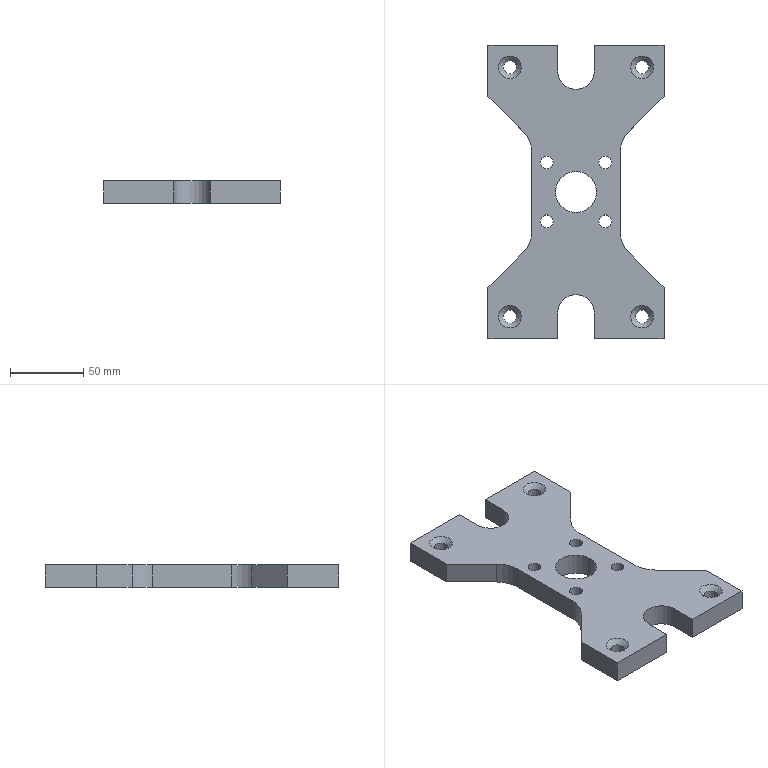Part | STEP file | 冲床-300配套压波_id762_x_t | 1 solid | 47 faces | box 120 x 200 x 15 mm | volume 229658 mm3 | plane 24 | cylinder 19 | cone 4 | commonest cylinder face diameters 8.7 x4 9 x4 14 x4 40 x4 25 x2 28 x1
STEP:
#1=CARTESIAN_POINT('',(1854.5,-85.,203.));
#2=VERTEX_POINT('',#1);
#3=CARTESIAN_POINT('',(1850.,-85.,203.));
#4=DIRECTION('',(0.,0.,1.));
#5=DIRECTION('',(1.,0.,0.));
#6=AXIS2_PLACEMENT_3D('',#3,#4,#5);
#7=CIRCLE('',#6,4.5);
#8=EDGE_CURVE('',#2,#2,#7,.T.);
#9=ORIENTED_EDGE('',*,*,#8,.F.);
#10=EDGE_LOOP('',(#9));
#11=FACE_BOUND('',#10,.T.);
#12=CARTESIAN_POINT('',(1854.5,-85.,214.78));
#13=VERTEX_POINT('',#12);
#14=CARTESIAN_POINT('',(1850.,-85.,214.78));
#15=DIRECTION('',(0.,0.,-1.));
#16=DIRECTION('',(1.,0.,0.));
#17=AXIS2_PLACEMENT_3D('',#14,#15,#16);
#18=CIRCLE('',#17,4.5);
#19=EDGE_CURVE('',#13,#13,#18,.T.);
#20=ORIENTED_EDGE('',*,*,#19,.F.);
#21=EDGE_LOOP('',(#20));
#22=FACE_BOUND('',#21,.T.);
#23=CARTESIAN_POINT('',(1850.,-85.,-72.));
#24=DIRECTION('',(0.,0.,1.));
#25=DIRECTION('',(1.,0.,0.));
#26=AXIS2_PLACEMENT_3D('',#23,#24,#25);
#27=CYLINDRICAL_SURFACE('',#26,4.5);
#28=ADVANCED_FACE('',(#11,#22),#27,.F.);
#29=CARTESIAN_POINT('',(1857.72,-85.,218.));
#30=VERTEX_POINT('',#29);
#31=CARTESIAN_POINT('',(1850.,-85.,218.));
#32=DIRECTION('',(0.,0.,-1.));
#33=DIRECTION('',(1.,0.,0.));
#34=AXIS2_PLACEMENT_3D('',#31,#32,#33);
#35=CIRCLE('',#34,7.72);
#36=EDGE_CURVE('',#30,#30,#35,.T.);
#37=ORIENTED_EDGE('',*,*,#36,.F.);
#38=EDGE_LOOP('',(#37));
#39=FACE_BOUND('',#38,.T.);
#40=ORIENTED_EDGE('',*,*,#19,.T.);
#41=EDGE_LOOP('',(#40));
#42=FACE_BOUND('',#41,.T.);
#43=CARTESIAN_POINT('',(1850.,-85.,215.95));
#44=DIRECTION('',(0.,0.,1.));
#45=DIRECTION('',(1.,0.,0.));
#46=AXIS2_PLACEMENT_3D('',#43,#44,#45);
#47=CONICAL_SURFACE('',#46,5.67,45.);
#48=ADVANCED_FACE('',(#39,#42),#47,.F.);
#49=CARTESIAN_POINT('',(1829.35,-20.,211.));
#50=VERTEX_POINT('',#49);
#51=CARTESIAN_POINT('',(1825.,-20.,211.));
#52=DIRECTION('',(0.,0.,1.));
#53=DIRECTION('',(1.,0.,0.));
#54=AXIS2_PLACEMENT_3D('',#51,#52,#53);
#55=CIRCLE('',#54,4.35);
#56=EDGE_CURVE('',#50,#50,#55,.T.);
#57=ORIENTED_EDGE('',*,*,#56,.T.);
#58=EDGE_LOOP('',(#57));
#59=FACE_BOUND('',#58,.T.);
#60=CARTESIAN_POINT('',(1832.,-20.,211.));
#61=VERTEX_POINT('',#60);
#62=CARTESIAN_POINT('',(1825.,-20.,211.));
#63=DIRECTION('',(0.,0.,-1.));
#64=DIRECTION('',(1.,0.,0.));
#65=AXIS2_PLACEMENT_3D('',#62,#63,#64);
#66=CIRCLE('',#65,7.);
#67=EDGE_CURVE('',#61,#61,#66,.T.);
#68=ORIENTED_EDGE('',*,*,#67,.T.);
#69=EDGE_LOOP('',(#68));
#70=FACE_BOUND('',#69,.T.);
#71=CARTESIAN_POINT('',(1825.,-20.,211.));
#72=DIRECTION('',(0.,0.,1.));
#73=DIRECTION('',(1.,0.,0.));
#74=AXIS2_PLACEMENT_3D('',#71,#72,#73);
#75=PLANE('',#74);
#76=ADVANCED_FACE('',(#59,#70),#75,.F.);
#77=CARTESIAN_POINT('',(1792.,20.,211.));
#78=VERTEX_POINT('',#77);
#79=CARTESIAN_POINT('',(1785.,20.,211.));
#80=DIRECTION('',(0.,0.,-1.));
#81=DIRECTION('',(1.,0.,0.));
#82=AXIS2_PLACEMENT_3D('',#79,#80,#81);
#83=CIRCLE('',#82,7.);
#84=EDGE_CURVE('',#78,#78,#83,.T.);
#85=ORIENTED_EDGE('',*,*,#84,.T.);
#86=EDGE_LOOP('',(#85));
#87=FACE_BOUND('',#86,.T.);
#88=CARTESIAN_POINT('',(1789.35,20.,211.));
#89=VERTEX_POINT('',#88);
#90=CARTESIAN_POINT('',(1785.,20.,211.));
#91=DIRECTION('',(0.,0.,-1.));
#92=DIRECTION('',(1.,0.,0.));
#93=AXIS2_PLACEMENT_3D('',#90,#91,#92);
#94=CIRCLE('',#93,4.35);
#95=EDGE_CURVE('',#89,#89,#94,.T.);
#96=ORIENTED_EDGE('',*,*,#95,.F.);
#97=EDGE_LOOP('',(#96));
#98=FACE_BOUND('',#97,.T.);
#99=CARTESIAN_POINT('',(1785.,20.,211.));
#100=DIRECTION('',(0.,0.,1.));
#101=DIRECTION('',(1.,0.,0.));
#102=AXIS2_PLACEMENT_3D('',#99,#100,#101);
#103=PLANE('',#102);
#104=ADVANCED_FACE('',(#87,#98),#103,.F.);
#105=CARTESIAN_POINT('',(1792.,-20.,211.));
#106=VERTEX_POINT('',#105);
#107=CARTESIAN_POINT('',(1785.,-20.,211.));
#108=DIRECTION('',(0.,0.,-1.));
#109=DIRECTION('',(1.,0.,0.));
#110=AXIS2_PLACEMENT_3D('',#107,#108,#109);
#111=CIRCLE('',#110,7.);
#112=EDGE_CURVE('',#106,#106,#111,.T.);
#113=ORIENTED_EDGE('',*,*,#112,.T.);
#114=EDGE_LOOP('',(#113));
#115=FACE_BOUND('',#114,.T.);
#116=CARTESIAN_POINT('',(1789.35,-20.,211.));
#117=VERTEX_POINT('',#116);
#118=CARTESIAN_POINT('',(1785.,-20.,211.));
#119=DIRECTION('',(0.,0.,-1.));
#120=DIRECTION('',(1.,0.,0.));
#121=AXIS2_PLACEMENT_3D('',#118,#119,#120);
#122=CIRCLE('',#121,4.35);
#123=EDGE_CURVE('',#117,#117,#122,.T.);
#124=ORIENTED_EDGE('',*,*,#123,.F.);
#125=EDGE_LOOP('',(#124));
#126=FACE_BOUND('',#125,.T.);
#127=CARTESIAN_POINT('',(1785.,-20.,211.));
#128=DIRECTION('',(0.,0.,1.));
#129=DIRECTION('',(1.,0.,0.));
#130=AXIS2_PLACEMENT_3D('',#127,#128,#129);
#131=PLANE('',#130);
#132=ADVANCED_FACE('',(#115,#126),#131,.F.);
#133=CARTESIAN_POINT('',(1832.,20.,211.));
#134=VERTEX_POINT('',#133);
#135=CARTESIAN_POINT('',(1825.,20.,211.));
#136=DIRECTION('',(0.,0.,-1.));
#137=DIRECTION('',(1.,0.,0.));
#138=AXIS2_PLACEMENT_3D('',#135,#136,#137);
#139=CIRCLE('',#138,7.);
#140=EDGE_CURVE('',#134,#134,#139,.T.);
#141=ORIENTED_EDGE('',*,*,#140,.T.);
#142=EDGE_LOOP('',(#141));
#143=FACE_BOUND('',#142,.T.);
#144=CARTESIAN_POINT('',(1829.35,20.,211.));
#145=VERTEX_POINT('',#144);
#146=CARTESIAN_POINT('',(1825.,20.,211.));
#147=DIRECTION('',(0.,0.,-1.));
#148=DIRECTION('',(1.,0.,0.));
#149=AXIS2_PLACEMENT_3D('',#146,#147,#148);
#150=CIRCLE('',#149,4.35);
#151=EDGE_CURVE('',#145,#145,#150,.T.);
#152=ORIENTED_EDGE('',*,*,#151,.F.);
#153=EDGE_LOOP('',(#152));
#154=FACE_BOUND('',#153,.T.);
#155=CARTESIAN_POINT('',(1825.,20.,211.));
#156=DIRECTION('',(0.,0.,1.));
#157=DIRECTION('',(1.,0.,0.));
#158=AXIS2_PLACEMENT_3D('',#155,#156,#157);
#159=PLANE('',#158);
#160=ADVANCED_FACE('',(#143,#154),#159,.F.);
#161=ORIENTED_EDGE('',*,*,#56,.F.);
#162=EDGE_LOOP('',(#161));
#163=FACE_BOUND('',#162,.T.);
#164=CARTESIAN_POINT('',(1829.35,-20.,218.));
#165=VERTEX_POINT('',#164);
#166=CARTESIAN_POINT('',(1825.,-20.,218.));
#167=DIRECTION('',(0.,0.,-1.));
#168=DIRECTION('',(1.,0.,0.));
#169=AXIS2_PLACEMENT_3D('',#166,#167,#168);
#170=CIRCLE('',#169,4.35);
#171=EDGE_CURVE('',#165,#165,#170,.T.);
#172=ORIENTED_EDGE('',*,*,#171,.F.);
#173=EDGE_LOOP('',(#172));
#174=FACE_BOUND('',#173,.T.);
#175=CARTESIAN_POINT('',(1825.,-20.,186.));
#176=DIRECTION('',(0.,0.,1.));
#177=DIRECTION('',(1.,0.,0.));
#178=AXIS2_PLACEMENT_3D('',#175,#176,#177);
#179=CYLINDRICAL_SURFACE('',#178,4.35);
#180=ADVANCED_FACE('',(#163,#174),#179,.F.);
#181=ORIENTED_EDGE('',*,*,#95,.T.);
#182=EDGE_LOOP('',(#181));
#183=FACE_BOUND('',#182,.T.);
#184=CARTESIAN_POINT('',(1789.35,20.,218.));
#185=VERTEX_POINT('',#184);
#186=CARTESIAN_POINT('',(1785.,20.,218.));
#187=DIRECTION('',(0.,0.,1.));
#188=DIRECTION('',(1.,0.,0.));
#189=AXIS2_PLACEMENT_3D('',#186,#187,#188);
#190=CIRCLE('',#189,4.35);
#191=EDGE_CURVE('',#185,#185,#190,.T.);
#192=ORIENTED_EDGE('',*,*,#191,.T.);
#193=EDGE_LOOP('',(#192));
#194=FACE_BOUND('',#193,.T.);
#195=CARTESIAN_POINT('',(1785.,20.,186.));
#196=DIRECTION('',(0.,0.,1.));
#197=DIRECTION('',(1.,0.,0.));
#198=AXIS2_PLACEMENT_3D('',#195,#196,#197);
#199=CYLINDRICAL_SURFACE('',#198,4.35);
#200=ADVANCED_FACE('',(#183,#194),#199,.F.);
#201=ORIENTED_EDGE('',*,*,#123,.T.);
#202=EDGE_LOOP('',(#201));
#203=FACE_BOUND('',#202,.T.);
#204=CARTESIAN_POINT('',(1789.35,-20.,218.));
#205=VERTEX_POINT('',#204);
#206=CARTESIAN_POINT('',(1785.,-20.,218.));
#207=DIRECTION('',(0.,0.,1.));
#208=DIRECTION('',(1.,0.,0.));
#209=AXIS2_PLACEMENT_3D('',#206,#207,#208);
#210=CIRCLE('',#209,4.35);
#211=EDGE_CURVE('',#205,#205,#210,.T.);
#212=ORIENTED_EDGE('',*,*,#211,.T.);
#213=EDGE_LOOP('',(#212));
#214=FACE_BOUND('',#213,.T.);
#215=CARTESIAN_POINT('',(1785.,-20.,186.));
#216=DIRECTION('',(0.,0.,1.));
#217=DIRECTION('',(1.,0.,0.));
#218=AXIS2_PLACEMENT_3D('',#215,#216,#217);
#219=CYLINDRICAL_SURFACE('',#218,4.35);
#220=ADVANCED_FACE('',(#203,#214),#219,.F.);
#221=ORIENTED_EDGE('',*,*,#151,.T.);
#222=EDGE_LOOP('',(#221));
#223=FACE_BOUND('',#222,.T.);
#224=CARTESIAN_POINT('',(1829.35,20.,218.));
#225=VERTEX_POINT('',#224);
#226=CARTESIAN_POINT('',(1825.,20.,218.));
#227=DIRECTION('',(0.,0.,1.));
#228=DIRECTION('',(1.,0.,0.));
#229=AXIS2_PLACEMENT_3D('',#226,#227,#228);
#230=CIRCLE('',#229,4.35);
#231=EDGE_CURVE('',#225,#225,#230,.T.);
#232=ORIENTED_EDGE('',*,*,#231,.T.);
#233=EDGE_LOOP('',(#232));
#234=FACE_BOUND('',#233,.T.);
#235=CARTESIAN_POINT('',(1825.,20.,186.));
#236=DIRECTION('',(0.,0.,1.));
#237=DIRECTION('',(1.,0.,0.));
#238=AXIS2_PLACEMENT_3D('',#235,#236,#237);
#239=CYLINDRICAL_SURFACE('',#238,4.35);
#240=ADVANCED_FACE('',(#223,#234),#239,.F.);
#241=CARTESIAN_POINT('',(1819.,0.,218.));
#242=VERTEX_POINT('',#241);
#243=CARTESIAN_POINT('',(1805.,0.,218.));
#244=DIRECTION('',(0.,0.,1.));
#245=DIRECTION('',(1.,0.,0.));
#246=AXIS2_PLACEMENT_3D('',#243,#244,#245);
#247=CIRCLE('',#246,14.);
#248=EDGE_CURVE('',#242,#242,#247,.T.);
#249=ORIENTED_EDGE('',*,*,#248,.T.);
#250=EDGE_LOOP('',(#249));
#251=FACE_BOUND('',#250,.T.);
#252=CARTESIAN_POINT('',(1819.,0.,203.));
#253=VERTEX_POINT('',#252);
#254=CARTESIAN_POINT('',(1805.,0.,203.));
#255=DIRECTION('',(0.,0.,1.));
#256=DIRECTION('',(1.,0.,0.));
#257=AXIS2_PLACEMENT_3D('',#254,#255,#256);
#258=CIRCLE('',#257,14.);
#259=EDGE_CURVE('',#253,#253,#258,.T.);
#260=ORIENTED_EDGE('',*,*,#259,.F.);
#261=EDGE_LOOP('',(#260));
#262=FACE_BOUND('',#261,.T.);
#263=CARTESIAN_POINT('',(1805.,0.,165.));
#264=DIRECTION('',(0.,0.,1.));
#265=DIRECTION('',(1.,0.,0.));
#266=AXIS2_PLACEMENT_3D('',#263,#264,#265);
#267=CYLINDRICAL_SURFACE('',#266,14.);
#268=ADVANCED_FACE('',(#251,#262),#267,.F.);
#269=CARTESIAN_POINT('',(1769.142,40.858,218.));
#270=VERTEX_POINT('',#269);
#271=CARTESIAN_POINT('',(1775.,26.716,218.));
#272=VERTEX_POINT('',#271);
#273=CARTESIAN_POINT('',(1755.,26.716,218.));
#274=DIRECTION('',(0.,0.,-1.));
#275=DIRECTION('',(1.,0.,0.));
#276=AXIS2_PLACEMENT_3D('',#273,#274,#275);
#277=CIRCLE('',#276,20.);
#278=EDGE_CURVE('',#270,#272,#277,.T.);
#279=ORIENTED_EDGE('',*,*,#278,.F.);
#280=CARTESIAN_POINT('',(1769.142,40.858,203.));
#281=VERTEX_POINT('',#280);
#282=CARTESIAN_POINT('',(1769.142,40.858,218.));
#283=DIRECTION('',(0.,0.,1.));
#284=VECTOR('',#283,1.);
#285=LINE('',#282,#284);
#286=EDGE_CURVE('',#281,#270,#285,.T.);
#287=ORIENTED_EDGE('',*,*,#286,.F.);
#288=CARTESIAN_POINT('',(1775.,26.716,203.));
#289=VERTEX_POINT('',#288);
#290=CARTESIAN_POINT('',(1755.,26.716,203.));
#291=DIRECTION('',(0.,0.,1.));
#292=DIRECTION('',(1.,0.,0.));
#293=AXIS2_PLACEMENT_3D('',#290,#291,#292);
#294=CIRCLE('',#293,20.);
#295=EDGE_CURVE('',#289,#281,#294,.T.);
#296=ORIENTED_EDGE('',*,*,#295,.F.);
#297=CARTESIAN_POINT('',(1775.,26.716,203.));
#298=DIRECTION('',(0.,0.,-1.));
#299=VECTOR('',#298,1.);
#300=LINE('',#297,#299);
#301=EDGE_CURVE('',#272,#289,#300,.T.);
#302=ORIENTED_EDGE('',*,*,#301,.F.);
#303=EDGE_LOOP('',(#279,#287,#296,#302));
#304=FACE_OUTER_BOUND('',#303,.T.);
#305=CARTESIAN_POINT('',(1755.,26.716,53.));
#306=DIRECTION('',(0.,0.,-1.));
#307=DIRECTION('',(-1.,0.,0.));
#308=AXIS2_PLACEMENT_3D('',#305,#306,#307);
#309=CYLINDRICAL_SURFACE('',#308,20.);
#310=ADVANCED_FACE('',(#304),#309,.F.);
#311=CARTESIAN_POINT('',(1745.,65.,203.));
#312=VERTEX_POINT('',#311);
#313=CARTESIAN_POINT('',(935.,875.,203.));
#314=DIRECTION('',(-0.7071,0.7071,0.));
#315=VECTOR('',#314,1.);
#316=LINE('',#313,#315);
#317=EDGE_CURVE('',#281,#312,#316,.T.);
#318=ORIENTED_EDGE('',*,*,#317,.F.);
#319=ORIENTED_EDGE('',*,*,#286,.T.);
#320=CARTESIAN_POINT('',(1745.,65.,218.));
#321=VERTEX_POINT('',#320);
#322=CARTESIAN_POINT('',(936.25,873.75,218.));
#323=DIRECTION('',(-0.7071,0.7071,0.));
#324=VECTOR('',#323,1.);
#325=LINE('',#322,#324);
#326=EDGE_CURVE('',#270,#321,#325,.T.);
#327=ORIENTED_EDGE('',*,*,#326,.T.);
#328=CARTESIAN_POINT('',(1745.,65.,113.));
#329=DIRECTION('',(0.,0.,1.));
#330=VECTOR('',#329,1.);
#331=LINE('',#328,#330);
#332=EDGE_CURVE('',#312,#321,#331,.T.);
#333=ORIENTED_EDGE('',*,*,#332,.F.);
#334=EDGE_LOOP('',(#318,#319,#327,#333));
#335=FACE_OUTER_BOUND('',#334,.T.);
#336=CARTESIAN_POINT('',(1745.,65.,113.));
#337=DIRECTION('',(-0.7071,-0.7071,0.));
#338=DIRECTION('',(0.,0.,-1.));
#339=AXIS2_PLACEMENT_3D('',#336,#337,#338);
#340=PLANE('',#339);
#341=ADVANCED_FACE('',(#335),#340,.T.);
#342=CARTESIAN_POINT('',(1745.,100.,203.));
#343=VERTEX_POINT('',#342);
#344=CARTESIAN_POINT('',(1745.,-60.,203.));
#345=DIRECTION('',(0.,-1.,0.));
#346=VECTOR('',#345,1.);
#347=LINE('',#344,#346);
#348=EDGE_CURVE('',#343,#312,#347,.T.);
#349=ORIENTED_EDGE('',*,*,#348,.T.);
#350=ORIENTED_EDGE('',*,*,#332,.T.);
#351=CARTESIAN_POINT('',(1745.,100.,218.));
#352=VERTEX_POINT('',#351);
#353=CARTESIAN_POINT('',(1745.,-60.,218.));
#354=DIRECTION('',(0.,-1.,0.));
#355=VECTOR('',#354,1.);
#356=LINE('',#353,#355);
#357=EDGE_CURVE('',#352,#321,#356,.T.);
#358=ORIENTED_EDGE('',*,*,#357,.F.);
#359=CARTESIAN_POINT('',(1745.,100.,113.));
#360=DIRECTION('',(0.,0.,-1.));
#361=VECTOR('',#360,1.);
#362=LINE('',#359,#361);
#363=EDGE_CURVE('',#352,#343,#362,.T.);
#364=ORIENTED_EDGE('',*,*,#363,.T.);
#365=EDGE_LOOP('',(#349,#350,#358,#364));
#366=FACE_OUTER_BOUND('',#365,.T.);
#367=CARTESIAN_POINT('',(1745.,-60.,113.));
#368=DIRECTION('',(-1.,0.,0.));
#369=DIRECTION('',(0.,0.,1.));
#370=AXIS2_PLACEMENT_3D('',#367,#368,#369);
#371=PLANE('',#370);
#372=ADVANCED_FACE('',(#366),#371,.T.);
#373=CARTESIAN_POINT('',(1792.5,100.,218.));
#374=VERTEX_POINT('',#373);
#375=CARTESIAN_POINT('',(1895.,100.,218.));
#376=DIRECTION('',(-1.,0.,0.));
#377=VECTOR('',#376,1.);
#378=LINE('',#375,#377);
#379=EDGE_CURVE('',#374,#352,#378,.T.);
#380=ORIENTED_EDGE('',*,*,#379,.F.);
#381=CARTESIAN_POINT('',(1792.5,100.,203.));
#382=VERTEX_POINT('',#381);
#383=CARTESIAN_POINT('',(1792.5,100.,318.));
#384=DIRECTION('',(0.,0.,-1.));
#385=VECTOR('',#384,1.);
#386=LINE('',#383,#385);
#387=EDGE_CURVE('',#374,#382,#386,.T.);
#388=ORIENTED_EDGE('',*,*,#387,.T.);
#389=CARTESIAN_POINT('',(1895.,100.,203.));
#390=DIRECTION('',(-1.,0.,0.));
#391=VECTOR('',#390,1.);
#392=LINE('',#389,#391);
#393=EDGE_CURVE('',#382,#343,#392,.T.);
#394=ORIENTED_EDGE('',*,*,#393,.T.);
#395=ORIENTED_EDGE('',*,*,#363,.F.);
#396=EDGE_LOOP('',(#380,#388,#394,#395));
#397=FACE_OUTER_BOUND('',#396,.T.);
#398=CARTESIAN_POINT('',(1895.,100.,318.));
#399=DIRECTION('',(0.,-1.,0.));
#400=DIRECTION('',(0.,0.,-1.));
#401=AXIS2_PLACEMENT_3D('',#398,#399,#400);
#402=PLANE('',#401);
#403=ADVANCED_FACE('',(#397),#402,.F.);
#404=CARTESIAN_POINT('',(1792.5,82.5,203.));
#405=VERTEX_POINT('',#404);
#406=CARTESIAN_POINT('',(1792.5,0.,203.));
#407=DIRECTION('',(0.,-1.,0.));
#408=VECTOR('',#407,1.);
#409=LINE('',#406,#408);
#410=EDGE_CURVE('',#382,#405,#409,.T.);
#411=ORIENTED_EDGE('',*,*,#410,.F.);
#412=ORIENTED_EDGE('',*,*,#387,.F.);
#413=CARTESIAN_POINT('',(1792.5,82.5,218.));
#414=VERTEX_POINT('',#413);
#415=CARTESIAN_POINT('',(1792.5,0.,218.));
#416=DIRECTION('',(0.,1.,0.));
#417=VECTOR('',#416,1.);
#418=LINE('',#415,#417);
#419=EDGE_CURVE('',#414,#374,#418,.T.);
#420=ORIENTED_EDGE('',*,*,#419,.F.);
#421=CARTESIAN_POINT('',(1792.5,82.5,218.));
#422=DIRECTION('',(0.,0.,-1.));
#423=VECTOR('',#422,1.);
#424=LINE('',#421,#423);
#425=EDGE_CURVE('',#414,#405,#424,.T.);
#426=ORIENTED_EDGE('',*,*,#425,.T.);
#427=EDGE_LOOP('',(#411,#412,#420,#426));
#428=FACE_OUTER_BOUND('',#427,.T.);
#429=CARTESIAN_POINT('',(1792.5,70.,18.));
#430=DIRECTION('',(-1.,0.,0.));
#431=DIRECTION('',(0.,0.,1.));
#432=AXIS2_PLACEMENT_3D('',#429,#430,#431);
#433=PLANE('',#432);
#434=ADVANCED_FACE('',(#428),#433,.F.);
#435=CARTESIAN_POINT('',(1817.5,82.5,218.));
#436=VERTEX_POINT('',#435);
#437=CARTESIAN_POINT('',(1805.,82.5,218.));
#438=DIRECTION('',(0.,0.,1.));
#439=DIRECTION('',(1.,0.,0.));
#440=AXIS2_PLACEMENT_3D('',#437,#438,#439);
#441=CIRCLE('',#440,12.5);
#442=EDGE_CURVE('',#414,#436,#441,.T.);
#443=ORIENTED_EDGE('',*,*,#442,.T.);
#444=CARTESIAN_POINT('',(1817.5,82.5,203.));
#445=VERTEX_POINT('',#444);
#446=CARTESIAN_POINT('',(1817.5,82.5,218.));
#447=DIRECTION('',(0.,0.,1.));
#448=VECTOR('',#447,1.);
#449=LINE('',#446,#448);
#450=EDGE_CURVE('',#445,#436,#449,.T.);
#451=ORIENTED_EDGE('',*,*,#450,.F.);
#452=CARTESIAN_POINT('',(1805.,82.5,203.));
#453=DIRECTION('',(0.,0.,1.));
#454=DIRECTION('',(1.,0.,0.));
#455=AXIS2_PLACEMENT_3D('',#452,#453,#454);
#456=CIRCLE('',#455,12.5);
#457=EDGE_CURVE('',#405,#445,#456,.T.);
#458=ORIENTED_EDGE('',*,*,#457,.F.);
#459=ORIENTED_EDGE('',*,*,#425,.F.);
#460=EDGE_LOOP('',(#443,#451,#458,#459));
#461=FACE_OUTER_BOUND('',#460,.T.);
#462=CARTESIAN_POINT('',(1805.,82.5,18.));
#463=DIRECTION('',(0.,0.,1.));
#464=DIRECTION('',(1.,0.,0.));
#465=AXIS2_PLACEMENT_3D('',#462,#463,#464);
#466=CYLINDRICAL_SURFACE('',#465,12.5);
#467=ADVANCED_FACE('',(#461),#466,.F.);
#468=CARTESIAN_POINT('',(1817.5,100.,203.));
#469=VERTEX_POINT('',#468);
#470=CARTESIAN_POINT('',(1817.5,0.,203.));
#471=DIRECTION('',(0.,1.,0.));
#472=VECTOR('',#471,1.);
#473=LINE('',#470,#472);
#474=EDGE_CURVE('',#445,#469,#473,.T.);
#475=ORIENTED_EDGE('',*,*,#474,.F.);
#476=ORIENTED_EDGE('',*,*,#450,.T.);
#477=CARTESIAN_POINT('',(1817.5,100.,218.));
#478=VERTEX_POINT('',#477);
#479=CARTESIAN_POINT('',(1817.5,0.,218.));
#480=DIRECTION('',(0.,-1.,0.));
#481=VECTOR('',#480,1.);
#482=LINE('',#479,#481);
#483=EDGE_CURVE('',#478,#436,#482,.T.);
#484=ORIENTED_EDGE('',*,*,#483,.F.);
#485=CARTESIAN_POINT('',(1817.5,100.,318.));
#486=DIRECTION('',(0.,0.,1.));
#487=VECTOR('',#486,1.);
#488=LINE('',#485,#487);
#489=EDGE_CURVE('',#469,#478,#488,.T.);
#490=ORIENTED_EDGE('',*,*,#489,.F.);
#491=EDGE_LOOP('',(#475,#476,#484,#490));
#492=FACE_OUTER_BOUND('',#491,.T.);
#493=CARTESIAN_POINT('',(1817.5,70.,18.));
#494=DIRECTION('',(1.,0.,0.));
#495=DIRECTION('',(0.,0.,1.));
#496=AXIS2_PLACEMENT_3D('',#493,#494,#495);
#497=PLANE('',#496);
#498=ADVANCED_FACE('',(#492),#497,.F.);
#499=CARTESIAN_POINT('',(1865.,100.,218.));
#500=VERTEX_POINT('',#499);
#501=CARTESIAN_POINT('',(1715.,100.,218.));
#502=DIRECTION('',(-1.,0.,0.));
#503=VECTOR('',#502,1.);
#504=LINE('',#501,#503);
#505=EDGE_CURVE('',#500,#478,#504,.T.);
#506=ORIENTED_EDGE('',*,*,#505,.F.);
#507=CARTESIAN_POINT('',(1865.,100.,203.));
#508=VERTEX_POINT('',#507);
#509=CARTESIAN_POINT('',(1865.,100.,113.));
#510=DIRECTION('',(0.,0.,1.));
#511=VECTOR('',#510,1.);
#512=LINE('',#509,#511);
#513=EDGE_CURVE('',#508,#500,#512,.T.);
#514=ORIENTED_EDGE('',*,*,#513,.F.);
#515=CARTESIAN_POINT('',(1715.,100.,203.));
#516=DIRECTION('',(-1.,0.,0.));
#517=VECTOR('',#516,1.);
#518=LINE('',#515,#517);
#519=EDGE_CURVE('',#508,#469,#518,.T.);
#520=ORIENTED_EDGE('',*,*,#519,.T.);
#521=ORIENTED_EDGE('',*,*,#489,.T.);
#522=EDGE_LOOP('',(#506,#514,#520,#521));
#523=FACE_OUTER_BOUND('',#522,.T.);
#524=CARTESIAN_POINT('',(1715.,100.,318.));
#525=DIRECTION('',(0.,-1.,0.));
#526=DIRECTION('',(0.,0.,-1.));
#527=AXIS2_PLACEMENT_3D('',#524,#525,#526);
#528=PLANE('',#527);
#529=ADVANCED_FACE('',(#523),#528,.F.);
#530=CARTESIAN_POINT('',(1865.,65.,203.));
#531=VERTEX_POINT('',#530);
#532=CARTESIAN_POINT('',(1865.,-60.,203.));
#533=DIRECTION('',(0.,1.,0.));
#534=VECTOR('',#533,1.);
#535=LINE('',#532,#534);
#536=EDGE_CURVE('',#531,#508,#535,.T.);
#537=ORIENTED_EDGE('',*,*,#536,.T.);
#538=ORIENTED_EDGE('',*,*,#513,.T.);
#539=CARTESIAN_POINT('',(1865.,65.,218.));
#540=VERTEX_POINT('',#539);
#541=CARTESIAN_POINT('',(1865.,-60.,218.));
#542=DIRECTION('',(0.,1.,0.));
#543=VECTOR('',#542,1.);
#544=LINE('',#541,#543);
#545=EDGE_CURVE('',#540,#500,#544,.T.);
#546=ORIENTED_EDGE('',*,*,#545,.F.);
#547=CARTESIAN_POINT('',(1865.,65.,113.));
#548=DIRECTION('',(0.,0.,-1.));
#549=VECTOR('',#548,1.);
#550=LINE('',#547,#549);
#551=EDGE_CURVE('',#540,#531,#550,.T.);
#552=ORIENTED_EDGE('',*,*,#551,.T.);
#553=EDGE_LOOP('',(#537,#538,#546,#552));
#554=FACE_OUTER_BOUND('',#553,.T.);
#555=CARTESIAN_POINT('',(1865.,-60.,113.));
#556=DIRECTION('',(1.,0.,0.));
#557=DIRECTION('',(0.,0.,1.));
#558=AXIS2_PLACEMENT_3D('',#555,#556,#557);
#559=PLANE('',#558);
#560=ADVANCED_FACE('',(#554),#559,.T.);
#561=CARTESIAN_POINT('',(1840.858,40.858,218.));
#562=VERTEX_POINT('',#561);
#563=CARTESIAN_POINT('',(2673.75,873.75,218.));
#564=DIRECTION('',(-0.7071,-0.7071,0.));
#565=VECTOR('',#564,1.);
#566=LINE('',#563,#565);
#567=EDGE_CURVE('',#540,#562,#566,.T.);
#568=ORIENTED_EDGE('',*,*,#567,.T.);
#569=CARTESIAN_POINT('',(1840.858,40.858,203.));
#570=VERTEX_POINT('',#569);
#571=CARTESIAN_POINT('',(1840.858,40.858,203.));
#572=DIRECTION('',(0.,0.,-1.));
#573=VECTOR('',#572,1.);
#574=LINE('',#571,#573);
#575=EDGE_CURVE('',#562,#570,#574,.T.);
#576=ORIENTED_EDGE('',*,*,#575,.T.);
#577=CARTESIAN_POINT('',(930.,-870.,203.));
#578=DIRECTION('',(-0.7071,-0.7071,0.));
#579=VECTOR('',#578,1.);
#580=LINE('',#577,#579);
#581=EDGE_CURVE('',#531,#570,#580,.T.);
#582=ORIENTED_EDGE('',*,*,#581,.F.);
#583=ORIENTED_EDGE('',*,*,#551,.F.);
#584=EDGE_LOOP('',(#568,#576,#582,#583));
#585=FACE_OUTER_BOUND('',#584,.T.);
#586=CARTESIAN_POINT('',(1865.,65.,113.));
#587=DIRECTION('',(0.7071,-0.7071,0.));
#588=DIRECTION('',(0.,0.,-1.));
#589=AXIS2_PLACEMENT_3D('',#586,#587,#588);
#590=PLANE('',#589);
#591=ADVANCED_FACE('',(#585),#590,.T.);
#592=CARTESIAN_POINT('',(1835.,26.716,203.));
#593=VERTEX_POINT('',#592);
#594=CARTESIAN_POINT('',(1855.,26.716,203.));
#595=DIRECTION('',(0.,0.,1.));
#596=DIRECTION('',(1.,0.,0.));
#597=AXIS2_PLACEMENT_3D('',#594,#595,#596);
#598=CIRCLE('',#597,20.);
#599=EDGE_CURVE('',#570,#593,#598,.T.);
#600=ORIENTED_EDGE('',*,*,#599,.F.);
#601=ORIENTED_EDGE('',*,*,#575,.F.);
#602=CARTESIAN_POINT('',(1835.,26.716,218.));
#603=VERTEX_POINT('',#602);
#604=CARTESIAN_POINT('',(1855.,26.716,218.));
#605=DIRECTION('',(0.,0.,-1.));
#606=DIRECTION('',(1.,0.,0.));
#607=AXIS2_PLACEMENT_3D('',#604,#605,#606);
#608=CIRCLE('',#607,20.);
#609=EDGE_CURVE('',#603,#562,#608,.T.);
#610=ORIENTED_EDGE('',*,*,#609,.F.);
#611=CARTESIAN_POINT('',(1835.,26.716,218.));
#612=DIRECTION('',(0.,0.,1.));
#613=VECTOR('',#612,1.);
#614=LINE('',#611,#613);
#615=EDGE_CURVE('',#593,#603,#614,.T.);
#616=ORIENTED_EDGE('',*,*,#615,.F.);
#617=EDGE_LOOP('',(#600,#601,#610,#616));
#618=FACE_OUTER_BOUND('',#617,.T.);
#619=CARTESIAN_POINT('',(1855.,26.716,53.));
#620=DIRECTION('',(0.,0.,1.));
#621=DIRECTION('',(1.,0.,0.));
#622=AXIS2_PLACEMENT_3D('',#619,#620,#621);
#623=CYLINDRICAL_SURFACE('',#622,20.);
#624=ADVANCED_FACE('',(#618),#623,.F.);
#625=CARTESIAN_POINT('',(1835.,-26.716,218.));
#626=VERTEX_POINT('',#625);
#627=CARTESIAN_POINT('',(1835.,0.,218.));
#628=DIRECTION('',(0.,-1.,0.));
#629=VECTOR('',#628,1.);
#630=LINE('',#627,#629);
#631=EDGE_CURVE('',#603,#626,#630,.T.);
#632=ORIENTED_EDGE('',*,*,#631,.T.);
#633=CARTESIAN_POINT('',(1835.,-26.716,203.));
#634=VERTEX_POINT('',#633);
#635=CARTESIAN_POINT('',(1835.,-26.716,203.));
#636=DIRECTION('',(0.,0.,-1.));
#637=VECTOR('',#636,1.);
#638=LINE('',#635,#637);
#639=EDGE_CURVE('',#626,#634,#638,.T.);
#640=ORIENTED_EDGE('',*,*,#639,.T.);
#641=CARTESIAN_POINT('',(1835.,0.,203.));
#642=DIRECTION('',(0.,-1.,0.));
#643=VECTOR('',#642,1.);
#644=LINE('',#641,#643);
#645=EDGE_CURVE('',#593,#634,#644,.T.);
#646=ORIENTED_EDGE('',*,*,#645,.F.);
#647=ORIENTED_EDGE('',*,*,#615,.T.);
#648=EDGE_LOOP('',(#632,#640,#646,#647));
#649=FACE_OUTER_BOUND('',#648,.T.);
#650=CARTESIAN_POINT('',(1835.,-50.,53.));
#651=DIRECTION('',(-1.,0.,0.));
#652=DIRECTION('',(0.,0.,-1.));
#653=AXIS2_PLACEMENT_3D('',#650,#651,#652);
#654=PLANE('',#653);
#655=ADVANCED_FACE('',(#649),#654,.F.);
#656=CARTESIAN_POINT('',(1840.858,-40.858,218.));
#657=VERTEX_POINT('',#656);
#658=CARTESIAN_POINT('',(1855.,-26.716,218.));
#659=DIRECTION('',(0.,0.,-1.));
#660=DIRECTION('',(1.,0.,0.));
#661=AXIS2_PLACEMENT_3D('',#658,#659,#660);
#662=CIRCLE('',#661,20.);
#663=EDGE_CURVE('',#657,#626,#662,.T.);
#664=ORIENTED_EDGE('',*,*,#663,.F.);
#665=CARTESIAN_POINT('',(1840.858,-40.858,203.));
#666=VERTEX_POINT('',#665);
#667=CARTESIAN_POINT('',(1840.858,-40.858,218.));
#668=DIRECTION('',(0.,0.,1.));
#669=VECTOR('',#668,1.);
#670=LINE('',#667,#669);
#671=EDGE_CURVE('',#666,#657,#670,.T.);
#672=ORIENTED_EDGE('',*,*,#671,.F.);
#673=CARTESIAN_POINT('',(1855.,-26.716,203.));
#674=DIRECTION('',(0.,0.,1.));
#675=DIRECTION('',(1.,0.,0.));
#676=AXIS2_PLACEMENT_3D('',#673,#674,#675);
#677=CIRCLE('',#676,20.);
#678=EDGE_CURVE('',#634,#666,#677,.T.);
#679=ORIENTED_EDGE('',*,*,#678,.F.);
#680=ORIENTED_EDGE('',*,*,#639,.F.);
#681=EDGE_LOOP('',(#664,#672,#679,#680));
#682=FACE_OUTER_BOUND('',#681,.T.);
#683=CARTESIAN_POINT('',(1855.,-26.716,53.));
#684=DIRECTION('',(0.,0.,-1.));
#685=DIRECTION('',(-1.,0.,0.));
#686=AXIS2_PLACEMENT_3D('',#683,#684,#685);
#687=CYLINDRICAL_SURFACE('',#686,20.);
#688=ADVANCED_FACE('',(#682),#687,.F.);
#689=CARTESIAN_POINT('',(1865.,-65.,203.));
#690=VERTEX_POINT('',#689);
#691=CARTESIAN_POINT('',(930.,870.,203.));
#692=DIRECTION('',(0.7071,-0.7071,0.));
#693=VECTOR('',#692,1.);
#694=LINE('',#691,#693);
#695=EDGE_CURVE('',#666,#690,#694,.T.);
#696=ORIENTED_EDGE('',*,*,#695,.F.);
#697=ORIENTED_EDGE('',*,*,#671,.T.);
#698=CARTESIAN_POINT('',(1865.,-65.,218.));
#699=VERTEX_POINT('',#698);
#700=CARTESIAN_POINT('',(2673.75,-873.75,218.));
#701=DIRECTION('',(0.7071,-0.7071,0.));
#702=VECTOR('',#701,1.);
#703=LINE('',#700,#702);
#704=EDGE_CURVE('',#657,#699,#703,.T.);
#705=ORIENTED_EDGE('',*,*,#704,.T.);
#706=CARTESIAN_POINT('',(1865.,-65.,113.));
#707=DIRECTION('',(0.,0.,1.));
#708=VECTOR('',#707,1.);
#709=LINE('',#706,#708);
#710=EDGE_CURVE('',#690,#699,#709,.T.);
#711=ORIENTED_EDGE('',*,*,#710,.F.);
#712=EDGE_LOOP('',(#696,#697,#705,#711));
#713=FACE_OUTER_BOUND('',#712,.T.);
#714=CARTESIAN_POINT('',(1865.,-65.,113.));
#715=DIRECTION('',(0.7071,0.7071,0.));
#716=DIRECTION('',(0.,0.,-1.));
#717=AXIS2_PLACEMENT_3D('',#714,#715,#716);
#718=PLANE('',#717);
#719=ADVANCED_FACE('',(#713),#718,.T.);
#720=CARTESIAN_POINT('',(1865.,-100.,203.));
#721=VERTEX_POINT('',#720);
#722=CARTESIAN_POINT('',(1865.,60.,203.));
#723=DIRECTION('',(0.,1.,0.));
#724=VECTOR('',#723,1.);
#725=LINE('',#722,#724);
#726=EDGE_CURVE('',#721,#690,#725,.T.);
#727=ORIENTED_EDGE('',*,*,#726,.T.);
#728=ORIENTED_EDGE('',*,*,#710,.T.);
#729=CARTESIAN_POINT('',(1865.,-100.,218.));
#730=VERTEX_POINT('',#729);
#731=CARTESIAN_POINT('',(1865.,60.,218.));
#732=DIRECTION('',(0.,1.,0.));
#733=VECTOR('',#732,1.);
#734=LINE('',#731,#733);
#735=EDGE_CURVE('',#730,#699,#734,.T.);
#736=ORIENTED_EDGE('',*,*,#735,.F.);
#737=CARTESIAN_POINT('',(1865.,-100.,113.));
#738=DIRECTION('',(0.,0.,-1.));
#739=VECTOR('',#738,1.);
#740=LINE('',#737,#739);
#741=EDGE_CURVE('',#730,#721,#740,.T.);
#742=ORIENTED_EDGE('',*,*,#741,.T.);
#743=EDGE_LOOP('',(#727,#728,#736,#742));
#744=FACE_OUTER_BOUND('',#743,.T.);
#745=CARTESIAN_POINT('',(1865.,60.,113.));
#746=DIRECTION('',(1.,0.,0.));
#747=DIRECTION('',(0.,0.,1.));
#748=AXIS2_PLACEMENT_3D('',#745,#746,#747);
#749=PLANE('',#748);
#750=ADVANCED_FACE('',(#744),#749,.T.);
#751=CARTESIAN_POINT('',(1817.5,-100.,218.));
#752=VERTEX_POINT('',#751);
#753=CARTESIAN_POINT('',(1715.,-100.,218.));
#754=DIRECTION('',(1.,0.,0.));
#755=VECTOR('',#754,1.);
#756=LINE('',#753,#755);
#757=EDGE_CURVE('',#752,#730,#756,.T.);
#758=ORIENTED_EDGE('',*,*,#757,.F.);
#759=CARTESIAN_POINT('',(1817.5,-100.,203.));
#760=VERTEX_POINT('',#759);
#761=CARTESIAN_POINT('',(1817.5,-100.,318.));
#762=DIRECTION('',(0.,0.,-1.));
#763=VECTOR('',#762,1.);
#764=LINE('',#761,#763);
#765=EDGE_CURVE('',#752,#760,#764,.T.);
#766=ORIENTED_EDGE('',*,*,#765,.T.);
#767=CARTESIAN_POINT('',(1715.,-100.,203.));
#768=DIRECTION('',(1.,0.,0.));
#769=VECTOR('',#768,1.);
#770=LINE('',#767,#769);
#771=EDGE_CURVE('',#760,#721,#770,.T.);
#772=ORIENTED_EDGE('',*,*,#771,.T.);
#773=ORIENTED_EDGE('',*,*,#741,.F.);
#774=EDGE_LOOP('',(#758,#766,#772,#773));
#775=FACE_OUTER_BOUND('',#774,.T.);
#776=CARTESIAN_POINT('',(1715.,-100.,318.));
#777=DIRECTION('',(0.,1.,0.));
#778=DIRECTION('',(0.,0.,-1.));
#779=AXIS2_PLACEMENT_3D('',#776,#777,#778);
#780=PLANE('',#779);
#781=ADVANCED_FACE('',(#775),#780,.F.);
#782=CARTESIAN_POINT('',(1817.5,-82.5,203.));
#783=VERTEX_POINT('',#782);
#784=CARTESIAN_POINT('',(1817.5,0.,203.));
#785=DIRECTION('',(0.,1.,0.));
#786=VECTOR('',#785,1.);
#787=LINE('',#784,#786);
#788=EDGE_CURVE('',#760,#783,#787,.T.);
#789=ORIENTED_EDGE('',*,*,#788,.F.);
#790=ORIENTED_EDGE('',*,*,#765,.F.);
#791=CARTESIAN_POINT('',(1817.5,-82.5,218.));
#792=VERTEX_POINT('',#791);
#793=CARTESIAN_POINT('',(1817.5,0.,218.));
#794=DIRECTION('',(0.,-1.,0.));
#795=VECTOR('',#794,1.);
#796=LINE('',#793,#795);
#797=EDGE_CURVE('',#792,#752,#796,.T.);
#798=ORIENTED_EDGE('',*,*,#797,.F.);
#799=CARTESIAN_POINT('',(1817.5,-82.5,218.));
#800=DIRECTION('',(0.,0.,-1.));
#801=VECTOR('',#800,1.);
#802=LINE('',#799,#801);
#803=EDGE_CURVE('',#792,#783,#802,.T.);
#804=ORIENTED_EDGE('',*,*,#803,.T.);
#805=EDGE_LOOP('',(#789,#790,#798,#804));
#806=FACE_OUTER_BOUND('',#805,.T.);
#807=CARTESIAN_POINT('',(1817.5,-70.,18.));
#808=DIRECTION('',(1.,0.,0.));
#809=DIRECTION('',(0.,0.,1.));
#810=AXIS2_PLACEMENT_3D('',#807,#808,#809);
#811=PLANE('',#810);
#812=ADVANCED_FACE('',(#806),#811,.F.);
#813=CARTESIAN_POINT('',(1792.5,-82.5,203.));
#814=VERTEX_POINT('',#813);
#815=CARTESIAN_POINT('',(1805.,-82.5,203.));
#816=DIRECTION('',(0.,0.,1.));
#817=DIRECTION('',(1.,0.,0.));
#818=AXIS2_PLACEMENT_3D('',#815,#816,#817);
#819=CIRCLE('',#818,12.5);
#820=EDGE_CURVE('',#783,#814,#819,.T.);
#821=ORIENTED_EDGE('',*,*,#820,.F.);
#822=ORIENTED_EDGE('',*,*,#803,.F.);
#823=CARTESIAN_POINT('',(1792.5,-82.5,218.));
#824=VERTEX_POINT('',#823);
#825=CARTESIAN_POINT('',(1805.,-82.5,218.));
#826=DIRECTION('',(0.,0.,1.));
#827=DIRECTION('',(1.,0.,0.));
#828=AXIS2_PLACEMENT_3D('',#825,#826,#827);
#829=CIRCLE('',#828,12.5);
#830=EDGE_CURVE('',#792,#824,#829,.T.);
#831=ORIENTED_EDGE('',*,*,#830,.T.);
#832=CARTESIAN_POINT('',(1792.5,-82.5,218.));
#833=DIRECTION('',(0.,0.,1.));
#834=VECTOR('',#833,1.);
#835=LINE('',#832,#834);
#836=EDGE_CURVE('',#814,#824,#835,.T.);
#837=ORIENTED_EDGE('',*,*,#836,.F.);
#838=EDGE_LOOP('',(#821,#822,#831,#837));
#839=FACE_OUTER_BOUND('',#838,.T.);
#840=CARTESIAN_POINT('',(1805.,-82.5,18.));
#841=DIRECTION('',(0.,0.,1.));
#842=DIRECTION('',(1.,0.,0.));
#843=AXIS2_PLACEMENT_3D('',#840,#841,#842);
#844=CYLINDRICAL_SURFACE('',#843,12.5);
#845=ADVANCED_FACE('',(#839),#844,.F.);
#846=CARTESIAN_POINT('',(1792.5,-100.,203.));
#847=VERTEX_POINT('',#846);
#848=CARTESIAN_POINT('',(1792.5,0.,203.));
#849=DIRECTION('',(0.,-1.,0.));
#850=VECTOR('',#849,1.);
#851=LINE('',#848,#850);
#852=EDGE_CURVE('',#814,#847,#851,.T.);
#853=ORIENTED_EDGE('',*,*,#852,.F.);
#854=ORIENTED_EDGE('',*,*,#836,.T.);
#855=CARTESIAN_POINT('',(1792.5,-100.,218.));
#856=VERTEX_POINT('',#855);
#857=CARTESIAN_POINT('',(1792.5,0.,218.));
#858=DIRECTION('',(0.,1.,0.));
#859=VECTOR('',#858,1.);
#860=LINE('',#857,#859);
#861=EDGE_CURVE('',#856,#824,#860,.T.);
#862=ORIENTED_EDGE('',*,*,#861,.F.);
#863=CARTESIAN_POINT('',(1792.5,-100.,318.));
#864=DIRECTION('',(0.,0.,1.));
#865=VECTOR('',#864,1.);
#866=LINE('',#863,#865);
#867=EDGE_CURVE('',#847,#856,#866,.T.);
#868=ORIENTED_EDGE('',*,*,#867,.F.);
#869=EDGE_LOOP('',(#853,#854,#862,#868));
#870=FACE_OUTER_BOUND('',#869,.T.);
#871=CARTESIAN_POINT('',(1792.5,-70.,18.));
#872=DIRECTION('',(-1.,0.,0.));
#873=DIRECTION('',(0.,0.,1.));
#874=AXIS2_PLACEMENT_3D('',#871,#872,#873);
#875=PLANE('',#874);
#876=ADVANCED_FACE('',(#870),#875,.F.);
#877=CARTESIAN_POINT('',(1745.,-100.,218.));
#878=VERTEX_POINT('',#877);
#879=CARTESIAN_POINT('',(1895.,-100.,218.));
#880=DIRECTION('',(1.,0.,0.));
#881=VECTOR('',#880,1.);
#882=LINE('',#879,#881);
#883=EDGE_CURVE('',#878,#856,#882,.T.);
#884=ORIENTED_EDGE('',*,*,#883,.F.);
#885=CARTESIAN_POINT('',(1745.,-100.,203.));
#886=VERTEX_POINT('',#885);
#887=CARTESIAN_POINT('',(1745.,-100.,113.));
#888=DIRECTION('',(0.,0.,1.));
#889=VECTOR('',#888,1.);
#890=LINE('',#887,#889);
#891=EDGE_CURVE('',#886,#878,#890,.T.);
#892=ORIENTED_EDGE('',*,*,#891,.F.);
#893=CARTESIAN_POINT('',(1895.,-100.,203.));
#894=DIRECTION('',(1.,0.,0.));
#895=VECTOR('',#894,1.);
#896=LINE('',#893,#895);
#897=EDGE_CURVE('',#886,#847,#896,.T.);
#898=ORIENTED_EDGE('',*,*,#897,.T.);
#899=ORIENTED_EDGE('',*,*,#867,.T.);
#900=EDGE_LOOP('',(#884,#892,#898,#899));
#901=FACE_OUTER_BOUND('',#900,.T.);
#902=CARTESIAN_POINT('',(1895.,-100.,318.));
#903=DIRECTION('',(0.,1.,0.));
#904=DIRECTION('',(0.,0.,-1.));
#905=AXIS2_PLACEMENT_3D('',#902,#903,#904);
#906=PLANE('',#905);
#907=ADVANCED_FACE('',(#901),#906,.F.);
#908=CARTESIAN_POINT('',(1745.,-65.,203.));
#909=VERTEX_POINT('',#908);
#910=CARTESIAN_POINT('',(1745.,60.,203.));
#911=DIRECTION('',(0.,-1.,0.));
#912=VECTOR('',#911,1.);
#913=LINE('',#910,#912);
#914=EDGE_CURVE('',#909,#886,#913,.T.);
#915=ORIENTED_EDGE('',*,*,#914,.T.);
#916=ORIENTED_EDGE('',*,*,#891,.T.);
#917=CARTESIAN_POINT('',(1745.,-65.,218.));
#918=VERTEX_POINT('',#917);
#919=CARTESIAN_POINT('',(1745.,60.,218.));
#920=DIRECTION('',(0.,-1.,0.));
#921=VECTOR('',#920,1.);
#922=LINE('',#919,#921);
#923=EDGE_CURVE('',#918,#878,#922,.T.);
#924=ORIENTED_EDGE('',*,*,#923,.F.);
#925=CARTESIAN_POINT('',(1745.,-65.,113.));
#926=DIRECTION('',(0.,0.,-1.));
#927=VECTOR('',#926,1.);
#928=LINE('',#925,#927);
#929=EDGE_CURVE('',#918,#909,#928,.T.);
#930=ORIENTED_EDGE('',*,*,#929,.T.);
#931=EDGE_LOOP('',(#915,#916,#924,#930));
#932=FACE_OUTER_BOUND('',#931,.T.);
#933=CARTESIAN_POINT('',(1745.,60.,113.));
#934=DIRECTION('',(-1.,0.,0.));
#935=DIRECTION('',(0.,0.,1.));
#936=AXIS2_PLACEMENT_3D('',#933,#934,#935);
#937=PLANE('',#936);
#938=ADVANCED_FACE('',(#932),#937,.T.);
#939=CARTESIAN_POINT('',(1769.142,-40.858,218.));
#940=VERTEX_POINT('',#939);
#941=CARTESIAN_POINT('',(936.25,-873.75,218.));
#942=DIRECTION('',(0.7071,0.7071,0.));
#943=VECTOR('',#942,1.);
#944=LINE('',#941,#943);
#945=EDGE_CURVE('',#918,#940,#944,.T.);
#946=ORIENTED_EDGE('',*,*,#945,.T.);
#947=CARTESIAN_POINT('',(1769.142,-40.858,203.));
#948=VERTEX_POINT('',#947);
#949=CARTESIAN_POINT('',(1769.142,-40.858,203.));
#950=DIRECTION('',(0.,0.,-1.));
#951=VECTOR('',#950,1.);
#952=LINE('',#949,#951);
#953=EDGE_CURVE('',#940,#948,#952,.T.);
#954=ORIENTED_EDGE('',*,*,#953,.T.);
#955=CARTESIAN_POINT('',(935.,-875.,203.));
#956=DIRECTION('',(0.7071,0.7071,0.));
#957=VECTOR('',#956,1.);
#958=LINE('',#955,#957);
#959=EDGE_CURVE('',#909,#948,#958,.T.);
#960=ORIENTED_EDGE('',*,*,#959,.F.);
#961=ORIENTED_EDGE('',*,*,#929,.F.);
#962=EDGE_LOOP('',(#946,#954,#960,#961));
#963=FACE_OUTER_BOUND('',#962,.T.);
#964=CARTESIAN_POINT('',(1745.,-65.,113.));
#965=DIRECTION('',(-0.7071,0.7071,0.));
#966=DIRECTION('',(0.,0.,-1.));
#967=AXIS2_PLACEMENT_3D('',#964,#965,#966);
#968=PLANE('',#967);
#969=ADVANCED_FACE('',(#963),#968,.T.);
#970=CARTESIAN_POINT('',(1775.,-26.716,203.));
#971=VERTEX_POINT('',#970);
#972=CARTESIAN_POINT('',(1755.,-26.716,203.));
#973=DIRECTION('',(0.,0.,1.));
#974=DIRECTION('',(1.,0.,0.));
#975=AXIS2_PLACEMENT_3D('',#972,#973,#974);
#976=CIRCLE('',#975,20.);
#977=EDGE_CURVE('',#948,#971,#976,.T.);
#978=ORIENTED_EDGE('',*,*,#977,.F.);
#979=ORIENTED_EDGE('',*,*,#953,.F.);
#980=CARTESIAN_POINT('',(1775.,-26.716,218.));
#981=VERTEX_POINT('',#980);
#982=CARTESIAN_POINT('',(1755.,-26.716,218.));
#983=DIRECTION('',(0.,0.,-1.));
#984=DIRECTION('',(1.,0.,0.));
#985=AXIS2_PLACEMENT_3D('',#982,#983,#984);
#986=CIRCLE('',#985,20.);
#987=EDGE_CURVE('',#981,#940,#986,.T.);
#988=ORIENTED_EDGE('',*,*,#987,.F.);
#989=CARTESIAN_POINT('',(1775.,-26.716,218.));
#990=DIRECTION('',(0.,0.,1.));
#991=VECTOR('',#990,1.);
#992=LINE('',#989,#991);
#993=EDGE_CURVE('',#971,#981,#992,.T.);
#994=ORIENTED_EDGE('',*,*,#993,.F.);
#995=EDGE_LOOP('',(#978,#979,#988,#994));
#996=FACE_OUTER_BOUND('',#995,.T.);
#997=CARTESIAN_POINT('',(1755.,-26.716,53.));
#998=DIRECTION('',(0.,0.,1.));
#999=DIRECTION('',(1.,0.,0.));
#1000=AXIS2_PLACEMENT_3D('',#997,#998,#999);
#1001=CYLINDRICAL_SURFACE('',#1000,20.);
#1002=ADVANCED_FACE('',(#996),#1001,.F.);
#1003=CARTESIAN_POINT('',(1775.,0.,203.));
#1004=DIRECTION('',(0.,1.,0.));
#1005=VECTOR('',#1004,1.);
#1006=LINE('',#1003,#1005);
#1007=EDGE_CURVE('',#971,#289,#1006,.T.);
#1008=ORIENTED_EDGE('',*,*,#1007,.F.);
#1009=ORIENTED_EDGE('',*,*,#993,.T.);
#1010=CARTESIAN_POINT('',(1775.,0.,218.));
#1011=DIRECTION('',(0.,1.,0.));
#1012=VECTOR('',#1011,1.);
#1013=LINE('',#1010,#1012);
#1014=EDGE_CURVE('',#981,#272,#1013,.T.);
#1015=ORIENTED_EDGE('',*,*,#1014,.T.);
#1016=ORIENTED_EDGE('',*,*,#301,.T.);
#1017=EDGE_LOOP('',(#1008,#1009,#1015,#1016));
#1018=FACE_OUTER_BOUND('',#1017,.T.);
#1019=CARTESIAN_POINT('',(1775.,50.,53.));
#1020=DIRECTION('',(1.,0.,0.));
#1021=DIRECTION('',(0.,0.,-1.));
#1022=AXIS2_PLACEMENT_3D('',#1019,#1020,#1021);
#1023=PLANE('',#1022);
#1024=ADVANCED_FACE('',(#1018),#1023,.F.);
#1025=CARTESIAN_POINT('',(1857.72,85.,218.));
#1026=VERTEX_POINT('',#1025);
#1027=CARTESIAN_POINT('',(1850.,85.,218.));
#1028=DIRECTION('',(0.,0.,1.));
#1029=DIRECTION('',(1.,0.,0.));
#1030=AXIS2_PLACEMENT_3D('',#1027,#1028,#1029);
#1031=CIRCLE('',#1030,7.72);
#1032=EDGE_CURVE('',#1026,#1026,#1031,.T.);
#1033=ORIENTED_EDGE('',*,*,#1032,.T.);
#1034=EDGE_LOOP('',(#1033));
#1035=FACE_BOUND('',#1034,.T.);
#1036=CARTESIAN_POINT('',(1854.5,85.,214.78));
#1037=VERTEX_POINT('',#1036);
#1038=CARTESIAN_POINT('',(1850.,85.,214.78));
#1039=DIRECTION('',(0.,0.,-1.));
#1040=DIRECTION('',(1.,0.,0.));
#1041=AXIS2_PLACEMENT_3D('',#1038,#1039,#1040);
#1042=CIRCLE('',#1041,4.5);
#1043=EDGE_CURVE('',#1037,#1037,#1042,.T.);
#1044=ORIENTED_EDGE('',*,*,#1043,.T.);
#1045=EDGE_LOOP('',(#1044));
#1046=FACE_BOUND('',#1045,.T.);
#1047=CARTESIAN_POINT('',(1850.,85.,215.95));
#1048=DIRECTION('',(0.,0.,1.));
#1049=DIRECTION('',(1.,0.,0.));
#1050=AXIS2_PLACEMENT_3D('',#1047,#1048,#1049);
#1051=CONICAL_SURFACE('',#1050,5.67,45.);
#1052=ADVANCED_FACE('',(#1035,#1046),#1051,.F.);
#1053=CARTESIAN_POINT('',(1752.28,85.,218.));
#1054=VERTEX_POINT('',#1053);
#1055=CARTESIAN_POINT('',(1760.,85.,218.));
#1056=DIRECTION('',(0.,0.,-1.));
#1057=DIRECTION('',(-1.,0.,0.));
#1058=AXIS2_PLACEMENT_3D('',#1055,#1056,#1057);
#1059=CIRCLE('',#1058,7.72);
#1060=EDGE_CURVE('',#1054,#1054,#1059,.T.);
#1061=ORIENTED_EDGE('',*,*,#1060,.F.);
#1062=EDGE_LOOP('',(#1061));
#1063=FACE_BOUND('',#1062,.T.);
#1064=CARTESIAN_POINT('',(1755.5,85.,214.78));
#1065=VERTEX_POINT('',#1064);
#1066=CARTESIAN_POINT('',(1760.,85.,214.78));
#1067=DIRECTION('',(0.,0.,-1.));
#1068=DIRECTION('',(-1.,0.,0.));
#1069=AXIS2_PLACEMENT_3D('',#1066,#1067,#1068);
#1070=CIRCLE('',#1069,4.5);
#1071=EDGE_CURVE('',#1065,#1065,#1070,.T.);
#1072=ORIENTED_EDGE('',*,*,#1071,.T.);
#1073=EDGE_LOOP('',(#1072));
#1074=FACE_BOUND('',#1073,.T.);
#1075=CARTESIAN_POINT('',(1760.,85.,215.95));
#1076=DIRECTION('',(0.,0.,1.));
#1077=DIRECTION('',(-1.,0.,0.));
#1078=AXIS2_PLACEMENT_3D('',#1075,#1076,#1077);
#1079=CONICAL_SURFACE('',#1078,5.67,45.);
#1080=ADVANCED_FACE('',(#1063,#1074),#1079,.F.);
#1081=CARTESIAN_POINT('',(1752.28,-85.,218.));
#1082=VERTEX_POINT('',#1081);
#1083=CARTESIAN_POINT('',(1760.,-85.,218.));
#1084=DIRECTION('',(0.,0.,-1.));
#1085=DIRECTION('',(-1.,0.,0.));
#1086=AXIS2_PLACEMENT_3D('',#1083,#1084,#1085);
#1087=CIRCLE('',#1086,7.72);
#1088=EDGE_CURVE('',#1082,#1082,#1087,.T.);
#1089=ORIENTED_EDGE('',*,*,#1088,.T.);
#1090=EDGE_LOOP('',(#1089));
#1091=FACE_BOUND('',#1090,.T.);
#1092=ORIENTED_EDGE('',*,*,#36,.T.);
#1093=EDGE_LOOP('',(#1092));
#1094=FACE_BOUND('',#1093,.T.);
#1095=ORIENTED_EDGE('',*,*,#1060,.T.);
#1096=EDGE_LOOP('',(#1095));
#1097=FACE_BOUND('',#1096,.T.);
#1098=ORIENTED_EDGE('',*,*,#1032,.F.);
#1099=EDGE_LOOP('',(#1098));
#1100=FACE_BOUND('',#1099,.T.);
#1101=ORIENTED_EDGE('',*,*,#1014,.F.);
#1102=ORIENTED_EDGE('',*,*,#987,.T.);
#1103=ORIENTED_EDGE('',*,*,#945,.F.);
#1104=ORIENTED_EDGE('',*,*,#923,.T.);
#1105=ORIENTED_EDGE('',*,*,#883,.T.);
#1106=ORIENTED_EDGE('',*,*,#861,.T.);
#1107=ORIENTED_EDGE('',*,*,#830,.F.);
#1108=ORIENTED_EDGE('',*,*,#797,.T.);
#1109=ORIENTED_EDGE('',*,*,#757,.T.);
#1110=ORIENTED_EDGE('',*,*,#735,.T.);
#1111=ORIENTED_EDGE('',*,*,#704,.F.);
#1112=ORIENTED_EDGE('',*,*,#663,.T.);
#1113=ORIENTED_EDGE('',*,*,#631,.F.);
#1114=ORIENTED_EDGE('',*,*,#609,.T.);
#1115=ORIENTED_EDGE('',*,*,#567,.F.);
#1116=ORIENTED_EDGE('',*,*,#545,.T.);
#1117=ORIENTED_EDGE('',*,*,#505,.T.);
#1118=ORIENTED_EDGE('',*,*,#483,.T.);
#1119=ORIENTED_EDGE('',*,*,#442,.F.);
#1120=ORIENTED_EDGE('',*,*,#419,.T.);
#1121=ORIENTED_EDGE('',*,*,#379,.T.);
#1122=ORIENTED_EDGE('',*,*,#357,.T.);
#1123=ORIENTED_EDGE('',*,*,#326,.F.);
#1124=ORIENTED_EDGE('',*,*,#278,.T.);
#1125=EDGE_LOOP('',(#1101,#1102,#1103,#1104,#1105,#1106,#1107,#1108,#1109,#1110,#1111,#1112,#1113,#1114,#1115,#1116,#1117,#1118,#1119,#1120,#1121,#1122,#1123,#1124));
#1126=FACE_BOUND('',#1125,.T.);
#1127=ORIENTED_EDGE('',*,*,#248,.F.);
#1128=EDGE_LOOP('',(#1127));
#1129=FACE_BOUND('',#1128,.T.);
#1130=ORIENTED_EDGE('',*,*,#231,.F.);
#1131=EDGE_LOOP('',(#1130));
#1132=FACE_BOUND('',#1131,.T.);
#1133=ORIENTED_EDGE('',*,*,#211,.F.);
#1134=EDGE_LOOP('',(#1133));
#1135=FACE_BOUND('',#1134,.T.);
#1136=ORIENTED_EDGE('',*,*,#191,.F.);
#1137=EDGE_LOOP('',(#1136));
#1138=FACE_BOUND('',#1137,.T.);
#1139=ORIENTED_EDGE('',*,*,#171,.T.);
#1140=EDGE_LOOP('',(#1139));
#1141=FACE_BOUND('',#1140,.T.);
#1142=CARTESIAN_POINT('',(60.,0.,218.));
#1143=DIRECTION('',(0.,0.,1.));
#1144=DIRECTION('',(1.,0.,0.));
#1145=AXIS2_PLACEMENT_3D('',#1142,#1143,#1144);
#1146=PLANE('',#1145);
#1147=ADVANCED_FACE('',(#1091,#1094,#1097,#1100,#1126,#1129,#1132,#1135,#1138,#1141),#1146,.T.);
#1148=CARTESIAN_POINT('',(1854.5,85.,203.));
#1149=VERTEX_POINT('',#1148);
#1150=CARTESIAN_POINT('',(1850.,85.,203.));
#1151=DIRECTION('',(0.,0.,1.));
#1152=DIRECTION('',(1.,0.,0.));
#1153=AXIS2_PLACEMENT_3D('',#1150,#1151,#1152);
#1154=CIRCLE('',#1153,4.5);
#1155=EDGE_CURVE('',#1149,#1149,#1154,.T.);
#1156=ORIENTED_EDGE('',*,*,#1155,.F.);
#1157=EDGE_LOOP('',(#1156));
#1158=FACE_BOUND('',#1157,.T.);
#1159=ORIENTED_EDGE('',*,*,#1043,.F.);
#1160=EDGE_LOOP('',(#1159));
#1161=FACE_BOUND('',#1160,.T.);
#1162=CARTESIAN_POINT('',(1850.,85.,-72.));
#1163=DIRECTION('',(0.,0.,1.));
#1164=DIRECTION('',(1.,0.,0.));
#1165=AXIS2_PLACEMENT_3D('',#1162,#1163,#1164);
#1166=CYLINDRICAL_SURFACE('',#1165,4.5);
#1167=ADVANCED_FACE('',(#1158,#1161),#1166,.F.);
#1168=ORIENTED_EDGE('',*,*,#140,.F.);
#1169=EDGE_LOOP('',(#1168));
#1170=FACE_BOUND('',#1169,.T.);
#1171=CARTESIAN_POINT('',(1832.,20.,203.));
#1172=VERTEX_POINT('',#1171);
#1173=CARTESIAN_POINT('',(1825.,20.,203.));
#1174=DIRECTION('',(0.,0.,1.));
#1175=DIRECTION('',(1.,0.,0.));
#1176=AXIS2_PLACEMENT_3D('',#1173,#1174,#1175);
#1177=CIRCLE('',#1176,7.);
#1178=EDGE_CURVE('',#1172,#1172,#1177,.T.);
#1179=ORIENTED_EDGE('',*,*,#1178,.F.);
#1180=EDGE_LOOP('',(#1179));
#1181=FACE_BOUND('',#1180,.T.);
#1182=CARTESIAN_POINT('',(1825.,20.,211.));
#1183=DIRECTION('',(0.,0.,-1.));
#1184=DIRECTION('',(-1.,0.,0.));
#1185=AXIS2_PLACEMENT_3D('',#1182,#1183,#1184);
#1186=CYLINDRICAL_SURFACE('',#1185,7.);
#1187=ADVANCED_FACE('',(#1170,#1181),#1186,.F.);
#1188=ORIENTED_EDGE('',*,*,#112,.F.);
#1189=EDGE_LOOP('',(#1188));
#1190=FACE_BOUND('',#1189,.T.);
#1191=CARTESIAN_POINT('',(1792.,-20.,203.));
#1192=VERTEX_POINT('',#1191);
#1193=CARTESIAN_POINT('',(1785.,-20.,203.));
#1194=DIRECTION('',(0.,0.,1.));
#1195=DIRECTION('',(1.,0.,0.));
#1196=AXIS2_PLACEMENT_3D('',#1193,#1194,#1195);
#1197=CIRCLE('',#1196,7.);
#1198=EDGE_CURVE('',#1192,#1192,#1197,.T.);
#1199=ORIENTED_EDGE('',*,*,#1198,.F.);
#1200=EDGE_LOOP('',(#1199));
#1201=FACE_BOUND('',#1200,.T.);
#1202=CARTESIAN_POINT('',(1785.,-20.,211.));
#1203=DIRECTION('',(0.,0.,-1.));
#1204=DIRECTION('',(-1.,0.,0.));
#1205=AXIS2_PLACEMENT_3D('',#1202,#1203,#1204);
#1206=CYLINDRICAL_SURFACE('',#1205,7.);
#1207=ADVANCED_FACE('',(#1190,#1201),#1206,.F.);
#1208=ORIENTED_EDGE('',*,*,#84,.F.);
#1209=EDGE_LOOP('',(#1208));
#1210=FACE_BOUND('',#1209,.T.);
#1211=CARTESIAN_POINT('',(1792.,20.,203.));
#1212=VERTEX_POINT('',#1211);
#1213=CARTESIAN_POINT('',(1785.,20.,203.));
#1214=DIRECTION('',(0.,0.,1.));
#1215=DIRECTION('',(1.,0.,0.));
#1216=AXIS2_PLACEMENT_3D('',#1213,#1214,#1215);
#1217=CIRCLE('',#1216,7.);
#1218=EDGE_CURVE('',#1212,#1212,#1217,.T.);
#1219=ORIENTED_EDGE('',*,*,#1218,.F.);
#1220=EDGE_LOOP('',(#1219));
#1221=FACE_BOUND('',#1220,.T.);
#1222=CARTESIAN_POINT('',(1785.,20.,211.));
#1223=DIRECTION('',(0.,0.,-1.));
#1224=DIRECTION('',(-1.,0.,0.));
#1225=AXIS2_PLACEMENT_3D('',#1222,#1223,#1224);
#1226=CYLINDRICAL_SURFACE('',#1225,7.);
#1227=ADVANCED_FACE('',(#1210,#1221),#1226,.F.);
#1228=ORIENTED_EDGE('',*,*,#67,.F.);
#1229=EDGE_LOOP('',(#1228));
#1230=FACE_BOUND('',#1229,.T.);
#1231=CARTESIAN_POINT('',(1832.,-20.,203.));
#1232=VERTEX_POINT('',#1231);
#1233=CARTESIAN_POINT('',(1825.,-20.,203.));
#1234=DIRECTION('',(0.,0.,1.));
#1235=DIRECTION('',(1.,0.,0.));
#1236=AXIS2_PLACEMENT_3D('',#1233,#1234,#1235);
#1237=CIRCLE('',#1236,7.);
#1238=EDGE_CURVE('',#1232,#1232,#1237,.T.);
#1239=ORIENTED_EDGE('',*,*,#1238,.F.);
#1240=EDGE_LOOP('',(#1239));
#1241=FACE_BOUND('',#1240,.T.);
#1242=CARTESIAN_POINT('',(1825.,-20.,211.));
#1243=DIRECTION('',(0.,0.,-1.));
#1244=DIRECTION('',(-1.,0.,0.));
#1245=AXIS2_PLACEMENT_3D('',#1242,#1243,#1244);
#1246=CYLINDRICAL_SURFACE('',#1245,7.);
#1247=ADVANCED_FACE('',(#1230,#1241),#1246,.F.);
#1248=CARTESIAN_POINT('',(1755.5,85.,203.));
#1249=VERTEX_POINT('',#1248);
#1250=CARTESIAN_POINT('',(1760.,85.,203.));
#1251=DIRECTION('',(0.,0.,1.));
#1252=DIRECTION('',(-1.,0.,0.));
#1253=AXIS2_PLACEMENT_3D('',#1250,#1251,#1252);
#1254=CIRCLE('',#1253,4.5);
#1255=EDGE_CURVE('',#1249,#1249,#1254,.T.);
#1256=ORIENTED_EDGE('',*,*,#1255,.F.);
#1257=EDGE_LOOP('',(#1256));
#1258=FACE_BOUND('',#1257,.T.);
#1259=ORIENTED_EDGE('',*,*,#1071,.F.);
#1260=EDGE_LOOP('',(#1259));
#1261=FACE_BOUND('',#1260,.T.);
#1262=CARTESIAN_POINT('',(1760.,85.,-72.));
#1263=DIRECTION('',(0.,0.,1.));
#1264=DIRECTION('',(-1.,0.,0.));
#1265=AXIS2_PLACEMENT_3D('',#1262,#1263,#1264);
#1266=CYLINDRICAL_SURFACE('',#1265,4.5);
#1267=ADVANCED_FACE('',(#1258,#1261),#1266,.F.);
#1268=CARTESIAN_POINT('',(1755.5,-85.,203.));
#1269=VERTEX_POINT('',#1268);
#1270=CARTESIAN_POINT('',(1760.,-85.,203.));
#1271=DIRECTION('',(0.,0.,1.));
#1272=DIRECTION('',(-1.,0.,0.));
#1273=AXIS2_PLACEMENT_3D('',#1270,#1271,#1272);
#1274=CIRCLE('',#1273,4.5);
#1275=EDGE_CURVE('',#1269,#1269,#1274,.T.);
#1276=ORIENTED_EDGE('',*,*,#1275,.T.);
#1277=EDGE_LOOP('',(#1276));
#1278=FACE_BOUND('',#1277,.T.);
#1279=ORIENTED_EDGE('',*,*,#8,.T.);
#1280=EDGE_LOOP('',(#1279));
#1281=FACE_BOUND('',#1280,.T.);
#1282=ORIENTED_EDGE('',*,*,#1255,.T.);
#1283=EDGE_LOOP('',(#1282));
#1284=FACE_BOUND('',#1283,.T.);
#1285=ORIENTED_EDGE('',*,*,#1238,.T.);
#1286=EDGE_LOOP('',(#1285));
#1287=FACE_BOUND('',#1286,.T.);
#1288=ORIENTED_EDGE('',*,*,#1218,.T.);
#1289=EDGE_LOOP('',(#1288));
#1290=FACE_BOUND('',#1289,.T.);
#1291=ORIENTED_EDGE('',*,*,#1198,.T.);
#1292=EDGE_LOOP('',(#1291));
#1293=FACE_BOUND('',#1292,.T.);
#1294=ORIENTED_EDGE('',*,*,#1178,.T.);
#1295=EDGE_LOOP('',(#1294));
#1296=FACE_BOUND('',#1295,.T.);
#1297=ORIENTED_EDGE('',*,*,#1155,.T.);
#1298=EDGE_LOOP('',(#1297));
#1299=FACE_BOUND('',#1298,.T.);
#1300=ORIENTED_EDGE('',*,*,#259,.T.);
#1301=EDGE_LOOP('',(#1300));
#1302=FACE_BOUND('',#1301,.T.);
#1303=ORIENTED_EDGE('',*,*,#959,.T.);
#1304=ORIENTED_EDGE('',*,*,#977,.T.);
#1305=ORIENTED_EDGE('',*,*,#1007,.T.);
#1306=ORIENTED_EDGE('',*,*,#295,.T.);
#1307=ORIENTED_EDGE('',*,*,#317,.T.);
#1308=ORIENTED_EDGE('',*,*,#348,.F.);
#1309=ORIENTED_EDGE('',*,*,#393,.F.);
#1310=ORIENTED_EDGE('',*,*,#410,.T.);
#1311=ORIENTED_EDGE('',*,*,#457,.T.);
#1312=ORIENTED_EDGE('',*,*,#474,.T.);
#1313=ORIENTED_EDGE('',*,*,#519,.F.);
#1314=ORIENTED_EDGE('',*,*,#536,.F.);
#1315=ORIENTED_EDGE('',*,*,#581,.T.);
#1316=ORIENTED_EDGE('',*,*,#599,.T.);
#1317=ORIENTED_EDGE('',*,*,#645,.T.);
#1318=ORIENTED_EDGE('',*,*,#678,.T.);
#1319=ORIENTED_EDGE('',*,*,#695,.T.);
#1320=ORIENTED_EDGE('',*,*,#726,.F.);
#1321=ORIENTED_EDGE('',*,*,#771,.F.);
#1322=ORIENTED_EDGE('',*,*,#788,.T.);
#1323=ORIENTED_EDGE('',*,*,#820,.T.);
#1324=ORIENTED_EDGE('',*,*,#852,.T.);
#1325=ORIENTED_EDGE('',*,*,#897,.F.);
#1326=ORIENTED_EDGE('',*,*,#914,.F.);
#1327=EDGE_LOOP('',(#1303,#1304,#1305,#1306,#1307,#1308,#1309,#1310,#1311,#1312,#1313,#1314,#1315,#1316,#1317,#1318,#1319,#1320,#1321,#1322,#1323,#1324,#1325,#1326));
#1328=FACE_BOUND('',#1327,.T.);
#1329=CARTESIAN_POINT('',(60.,0.,203.));
#1330=DIRECTION('',(0.,0.,1.));
#1331=DIRECTION('',(1.,0.,0.));
#1332=AXIS2_PLACEMENT_3D('',#1329,#1330,#1331);
#1333=PLANE('',#1332);
#1334=ADVANCED_FACE('',(#1278,#1281,#1284,#1287,#1290,#1293,#1296,#1299,#1302,#1328),#1333,.F.);
#1335=ORIENTED_EDGE('',*,*,#1275,.F.);
#1336=EDGE_LOOP('',(#1335));
#1337=FACE_BOUND('',#1336,.T.);
#1338=CARTESIAN_POINT('',(1755.5,-85.,214.78));
#1339=VERTEX_POINT('',#1338);
#1340=CARTESIAN_POINT('',(1760.,-85.,214.78));
#1341=DIRECTION('',(0.,0.,-1.));
#1342=DIRECTION('',(-1.,0.,0.));
#1343=AXIS2_PLACEMENT_3D('',#1340,#1341,#1342);
#1344=CIRCLE('',#1343,4.5);
#1345=EDGE_CURVE('',#1339,#1339,#1344,.T.);
#1346=ORIENTED_EDGE('',*,*,#1345,.F.);
#1347=EDGE_LOOP('',(#1346));
#1348=FACE_BOUND('',#1347,.T.);
#1349=CARTESIAN_POINT('',(1760.,-85.,-72.));
#1350=DIRECTION('',(0.,0.,1.));
#1351=DIRECTION('',(-1.,0.,0.));
#1352=AXIS2_PLACEMENT_3D('',#1349,#1350,#1351);
#1353=CYLINDRICAL_SURFACE('',#1352,4.5);
#1354=ADVANCED_FACE('',(#1337,#1348),#1353,.F.);
#1355=ORIENTED_EDGE('',*,*,#1088,.F.);
#1356=EDGE_LOOP('',(#1355));
#1357=FACE_BOUND('',#1356,.T.);
#1358=ORIENTED_EDGE('',*,*,#1345,.T.);
#1359=EDGE_LOOP('',(#1358));
#1360=FACE_BOUND('',#1359,.T.);
#1361=CARTESIAN_POINT('',(1760.,-85.,215.95));
#1362=DIRECTION('',(0.,0.,1.));
#1363=DIRECTION('',(-1.,0.,0.));
#1364=AXIS2_PLACEMENT_3D('',#1361,#1362,#1363);
#1365=CONICAL_SURFACE('',#1364,5.67,45.);
#1366=ADVANCED_FACE('',(#1357,#1360),#1365,.F.);
#1367=CLOSED_SHELL('',(#28,#48,#76,#104,#132,#160,#180,#200,#220,#240,#268,#310,#341,#372,#403,#434,#467,#498,#529,#560,#591,#624,#655,#688,#719,#750,#781,#812,#845,#876,#907,#938,#969,#1002,#1024,#1052,#1080,#1147,#1167,#1187,#1207,#1227,#1247,#1267,#1334,#1354,#1366));
#1368=MANIFOLD_SOLID_BREP('',#1367);
#1369=(LENGTH_UNIT()NAMED_UNIT(*)SI_UNIT(.MILLI.,.METRE.));
#1370=UNCERTAINTY_MEASURE_WITH_UNIT(LENGTH_MEASURE(0.00002),#1369,'','');
#1371=(NAMED_UNIT(*)PLANE_ANGLE_UNIT()SI_UNIT($,.RADIAN.));
#1372=PLANE_ANGLE_MEASURE_WITH_UNIT(PLANE_ANGLE_MEASURE(0.01745),#1371);
#1373=DIMENSIONAL_EXPONENTS(0.,0.,0.,0.,0.,0.,0.);
#1374=(CONVERSION_BASED_UNIT('DEGREE',#1372)NAMED_UNIT(#1373)PLANE_ANGLE_UNIT());
#1375=(NAMED_UNIT(*)SI_UNIT($,.STERADIAN.)SOLID_ANGLE_UNIT());
#1376=(GEOMETRIC_REPRESENTATION_CONTEXT(3)GLOBAL_UNCERTAINTY_ASSIGNED_CONTEXT((#1370))GLOBAL_UNIT_ASSIGNED_CONTEXT((#1369,#1374,#1375))REPRESENTATION_CONTEXT('',''));
#1377=ADVANCED_BREP_SHAPE_REPRESENTATION('',(#1368),#1376);